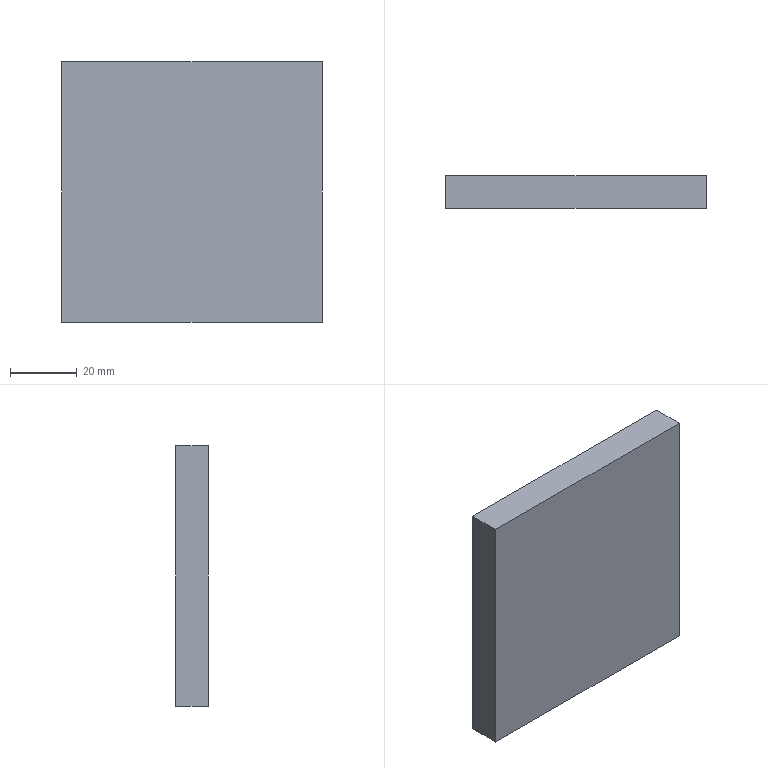Part | STEP file | 1 solid | 6 faces | box 77.948 x 9.733 x 78 mm | volume 59173 mm3 | plane 6
STEP:
#1=CARTESIAN_POINT('',(0.,0.,0.));
#2=DIRECTION('',(0.,0.,1.));
#3=DIRECTION('',(1.,0.,0.));
#4=AXIS2_PLACEMENT_3D('',#1,#2,#3);
#5=CARTESIAN_POINT('',(302.229,744.522,117.013));
#6=VERTEX_POINT('',#5);
#7=CARTESIAN_POINT('',(302.229,734.79,117.013));
#8=VERTEX_POINT('',#7);
#9=CARTESIAN_POINT('',(302.229,0.,117.013));
#10=DIRECTION('',(0.,-1.,0.));
#11=VECTOR('',#10,1.);
#12=LINE('',#9,#11);
#13=CARTESIAN_POINT('',(302.229,734.79,195.013));
#14=DIRECTION('',(1.,0.,0.));
#15=DIRECTION('',(0.,0.,-1.));
#16=AXIS2_PLACEMENT_3D('',#13,#14,#15);
#17=PLANE('',#16);
#18=CARTESIAN_POINT('',(78.,-734.79));
#19=DIRECTION('',(0.,-1.));
#20=VECTOR('',#19,1.);
#21=LINE('',#18,#20);
#22=(GEOMETRIC_REPRESENTATION_CONTEXT(2)PARAMETRIC_REPRESENTATION_CONTEXT()REPRESENTATION_CONTEXT('',''));
#23=DEFINITIONAL_REPRESENTATION('',(#21),#22);
#24=PCURVE('',#17,#23);
#25=CARTESIAN_POINT('',(0.,0.,117.013));
#26=DIRECTION('',(0.,0.,-1.));
#27=DIRECTION('',(-1.,0.,0.));
#28=AXIS2_PLACEMENT_3D('',#25,#26,#27);
#29=PLANE('',#28);
#30=CARTESIAN_POINT('',(-302.229,0.));
#31=DIRECTION('',(0.,-1.));
#32=VECTOR('',#31,1.);
#33=LINE('',#30,#32);
#34=(GEOMETRIC_REPRESENTATION_CONTEXT(2)PARAMETRIC_REPRESENTATION_CONTEXT()REPRESENTATION_CONTEXT('',''));
#35=DEFINITIONAL_REPRESENTATION('',(#33),#34);
#36=PCURVE('',#29,#35);
#37=SURFACE_CURVE('',#12,(#24,#36),.PCURVE_S1.);
#38=EDGE_CURVE('',#6,#8,#37,.T.);
#39=ORIENTED_EDGE('',*,*,#38,.T.);
#40=CARTESIAN_POINT('',(302.229,734.79,195.013));
#41=VERTEX_POINT('',#40);
#42=CARTESIAN_POINT('',(302.229,734.79,195.013));
#43=DIRECTION('',(0.,0.,-1.));
#44=VECTOR('',#43,1.);
#45=LINE('',#42,#44);
#46=CARTESIAN_POINT('',(0.,0.));
#47=DIRECTION('',(1.,0.));
#48=VECTOR('',#47,1.);
#49=LINE('',#46,#48);
#50=(GEOMETRIC_REPRESENTATION_CONTEXT(2)PARAMETRIC_REPRESENTATION_CONTEXT()REPRESENTATION_CONTEXT('',''));
#51=DEFINITIONAL_REPRESENTATION('',(#49),#50);
#52=PCURVE('',#17,#51);
#53=CARTESIAN_POINT('',(317.229,734.79,195.013));
#54=DIRECTION('',(0.,1.,0.));
#55=DIRECTION('',(0.,0.,1.));
#56=AXIS2_PLACEMENT_3D('',#53,#54,#55);
#57=PLANE('',#56);
#58=CARTESIAN_POINT('',(0.,-15.));
#59=DIRECTION('',(-1.,0.));
#60=VECTOR('',#59,1.);
#61=LINE('',#58,#60);
#62=(GEOMETRIC_REPRESENTATION_CONTEXT(2)PARAMETRIC_REPRESENTATION_CONTEXT()REPRESENTATION_CONTEXT('',''));
#63=DEFINITIONAL_REPRESENTATION('',(#61),#62);
#64=PCURVE('',#57,#63);
#65=SURFACE_CURVE('',#45,(#52,#64),.PCURVE_S1.);
#66=EDGE_CURVE('',#41,#8,#65,.T.);
#67=ORIENTED_EDGE('',*,*,#66,.F.);
#68=CARTESIAN_POINT('',(302.229,744.522,195.013));
#69=VERTEX_POINT('',#68);
#70=CARTESIAN_POINT('',(302.229,0.,195.013));
#71=DIRECTION('',(0.,-1.,0.));
#72=VECTOR('',#71,1.);
#73=LINE('',#70,#72);
#74=CARTESIAN_POINT('',(0.,-734.79));
#75=DIRECTION('',(0.,-1.));
#76=VECTOR('',#75,1.);
#77=LINE('',#74,#76);
#78=(GEOMETRIC_REPRESENTATION_CONTEXT(2)PARAMETRIC_REPRESENTATION_CONTEXT()REPRESENTATION_CONTEXT('',''));
#79=DEFINITIONAL_REPRESENTATION('',(#77),#78);
#80=PCURVE('',#17,#79);
#81=CARTESIAN_POINT('',(0.,0.,195.013));
#82=DIRECTION('',(0.,0.,-1.));
#83=DIRECTION('',(-1.,0.,0.));
#84=AXIS2_PLACEMENT_3D('',#81,#82,#83);
#85=PLANE('',#84);
#86=CARTESIAN_POINT('',(-302.229,0.));
#87=DIRECTION('',(0.,-1.));
#88=VECTOR('',#87,1.);
#89=LINE('',#86,#88);
#90=(GEOMETRIC_REPRESENTATION_CONTEXT(2)PARAMETRIC_REPRESENTATION_CONTEXT()REPRESENTATION_CONTEXT('',''));
#91=DEFINITIONAL_REPRESENTATION('',(#89),#90);
#92=PCURVE('',#85,#91);
#93=SURFACE_CURVE('',#73,(#80,#92),.PCURVE_S1.);
#94=EDGE_CURVE('',#69,#41,#93,.T.);
#95=ORIENTED_EDGE('',*,*,#94,.F.);
#96=CARTESIAN_POINT('',(302.229,744.522,195.013));
#97=DIRECTION('',(0.,0.,-1.));
#98=VECTOR('',#97,1.);
#99=LINE('',#96,#98);
#100=CARTESIAN_POINT('',(0.,9.733));
#101=DIRECTION('',(1.,0.));
#102=VECTOR('',#101,1.);
#103=LINE('',#100,#102);
#104=(GEOMETRIC_REPRESENTATION_CONTEXT(2)PARAMETRIC_REPRESENTATION_CONTEXT()REPRESENTATION_CONTEXT('',''));
#105=DEFINITIONAL_REPRESENTATION('',(#103),#104);
#106=PCURVE('',#17,#105);
#107=CARTESIAN_POINT('',(317.229,744.522,195.013));
#108=DIRECTION('',(0.,-1.,0.));
#109=DIRECTION('',(0.,0.,-1.));
#110=AXIS2_PLACEMENT_3D('',#107,#108,#109);
#111=PLANE('',#110);
#112=CARTESIAN_POINT('',(0.,-15.));
#113=DIRECTION('',(1.,0.));
#114=VECTOR('',#113,1.);
#115=LINE('',#112,#114);
#116=(GEOMETRIC_REPRESENTATION_CONTEXT(2)PARAMETRIC_REPRESENTATION_CONTEXT()REPRESENTATION_CONTEXT('',''));
#117=DEFINITIONAL_REPRESENTATION('',(#115),#116);
#118=PCURVE('',#111,#117);
#119=SURFACE_CURVE('',#99,(#106,#118),.PCURVE_S1.);
#120=EDGE_CURVE('',#69,#6,#119,.T.);
#121=ORIENTED_EDGE('',*,*,#120,.T.);
#122=EDGE_LOOP('',(#39,#67,#95,#121));
#123=FACE_BOUND('',#122,.T.);
#124=ADVANCED_FACE('',(#123),#17,.F.);
#125=CARTESIAN_POINT('',(380.177,734.79,117.013));
#126=VERTEX_POINT('',#125);
#127=CARTESIAN_POINT('',(0.,734.79,117.013));
#128=DIRECTION('',(1.,0.,0.));
#129=VECTOR('',#128,1.);
#130=LINE('',#127,#129);
#131=CARTESIAN_POINT('',(-78.,-317.229));
#132=DIRECTION('',(0.,1.));
#133=VECTOR('',#132,1.);
#134=LINE('',#131,#133);
#135=(GEOMETRIC_REPRESENTATION_CONTEXT(2)PARAMETRIC_REPRESENTATION_CONTEXT()REPRESENTATION_CONTEXT('',''));
#136=DEFINITIONAL_REPRESENTATION('',(#134),#135);
#137=PCURVE('',#57,#136);
#138=CARTESIAN_POINT('',(0.,734.79));
#139=DIRECTION('',(-1.,0.));
#140=VECTOR('',#139,1.);
#141=LINE('',#138,#140);
#142=(GEOMETRIC_REPRESENTATION_CONTEXT(2)PARAMETRIC_REPRESENTATION_CONTEXT()REPRESENTATION_CONTEXT('',''));
#143=DEFINITIONAL_REPRESENTATION('',(#141),#142);
#144=PCURVE('',#29,#143);
#145=SURFACE_CURVE('',#130,(#137,#144),.PCURVE_S1.);
#146=EDGE_CURVE('',#8,#126,#145,.T.);
#147=ORIENTED_EDGE('',*,*,#146,.T.);
#148=CARTESIAN_POINT('',(380.177,734.79,195.013));
#149=VERTEX_POINT('',#148);
#150=CARTESIAN_POINT('',(380.177,734.79,195.013));
#151=DIRECTION('',(0.,0.,-1.));
#152=VECTOR('',#151,1.);
#153=LINE('',#150,#152);
#154=CARTESIAN_POINT('',(0.,62.948));
#155=DIRECTION('',(-1.,0.));
#156=VECTOR('',#155,1.);
#157=LINE('',#154,#156);
#158=(GEOMETRIC_REPRESENTATION_CONTEXT(2)PARAMETRIC_REPRESENTATION_CONTEXT()REPRESENTATION_CONTEXT('',''));
#159=DEFINITIONAL_REPRESENTATION('',(#157),#158);
#160=PCURVE('',#57,#159);
#161=CARTESIAN_POINT('',(380.177,734.79,195.013));
#162=DIRECTION('',(-1.,0.,0.));
#163=DIRECTION('',(0.,0.,1.));
#164=AXIS2_PLACEMENT_3D('',#161,#162,#163);
#165=PLANE('',#164);
#166=CARTESIAN_POINT('',(0.,0.));
#167=DIRECTION('',(-1.,0.));
#168=VECTOR('',#167,1.);
#169=LINE('',#166,#168);
#170=(GEOMETRIC_REPRESENTATION_CONTEXT(2)PARAMETRIC_REPRESENTATION_CONTEXT()REPRESENTATION_CONTEXT('',''));
#171=DEFINITIONAL_REPRESENTATION('',(#169),#170);
#172=PCURVE('',#165,#171);
#173=SURFACE_CURVE('',#153,(#160,#172),.PCURVE_S1.);
#174=EDGE_CURVE('',#149,#126,#173,.T.);
#175=ORIENTED_EDGE('',*,*,#174,.F.);
#176=CARTESIAN_POINT('',(317.229,734.79,195.013));
#177=DIRECTION('',(1.,0.,0.));
#178=VECTOR('',#177,1.);
#179=LINE('',#176,#178);
#180=CARTESIAN_POINT('',(0.,0.));
#181=DIRECTION('',(0.,1.));
#182=VECTOR('',#181,1.);
#183=LINE('',#180,#182);
#184=(GEOMETRIC_REPRESENTATION_CONTEXT(2)PARAMETRIC_REPRESENTATION_CONTEXT()REPRESENTATION_CONTEXT('',''));
#185=DEFINITIONAL_REPRESENTATION('',(#183),#184);
#186=PCURVE('',#57,#185);
#187=CARTESIAN_POINT('',(-317.229,734.79));
#188=DIRECTION('',(-1.,0.));
#189=VECTOR('',#188,1.);
#190=LINE('',#187,#189);
#191=(GEOMETRIC_REPRESENTATION_CONTEXT(2)PARAMETRIC_REPRESENTATION_CONTEXT()REPRESENTATION_CONTEXT('',''));
#192=DEFINITIONAL_REPRESENTATION('',(#190),#191);
#193=PCURVE('',#85,#192);
#194=SURFACE_CURVE('',#179,(#186,#193),.PCURVE_S1.);
#195=EDGE_CURVE('',#41,#149,#194,.T.);
#196=ORIENTED_EDGE('',*,*,#195,.F.);
#197=ORIENTED_EDGE('',*,*,#66,.T.);
#198=EDGE_LOOP('',(#147,#175,#196,#197));
#199=FACE_BOUND('',#198,.T.);
#200=ADVANCED_FACE('',(#199),#57,.F.);
#201=CARTESIAN_POINT('',(380.177,744.522,117.013));
#202=VERTEX_POINT('',#201);
#203=CARTESIAN_POINT('',(380.177,0.,117.013));
#204=DIRECTION('',(0.,1.,0.));
#205=VECTOR('',#204,1.);
#206=LINE('',#203,#205);
#207=CARTESIAN_POINT('',(-78.,-734.79));
#208=DIRECTION('',(0.,1.));
#209=VECTOR('',#208,1.);
#210=LINE('',#207,#209);
#211=(GEOMETRIC_REPRESENTATION_CONTEXT(2)PARAMETRIC_REPRESENTATION_CONTEXT()REPRESENTATION_CONTEXT('',''));
#212=DEFINITIONAL_REPRESENTATION('',(#210),#211);
#213=PCURVE('',#165,#212);
#214=CARTESIAN_POINT('',(-380.177,0.));
#215=DIRECTION('',(0.,1.));
#216=VECTOR('',#215,1.);
#217=LINE('',#214,#216);
#218=(GEOMETRIC_REPRESENTATION_CONTEXT(2)PARAMETRIC_REPRESENTATION_CONTEXT()REPRESENTATION_CONTEXT('',''));
#219=DEFINITIONAL_REPRESENTATION('',(#217),#218);
#220=PCURVE('',#29,#219);
#221=SURFACE_CURVE('',#206,(#213,#220),.PCURVE_S1.);
#222=EDGE_CURVE('',#126,#202,#221,.T.);
#223=ORIENTED_EDGE('',*,*,#222,.T.);
#224=CARTESIAN_POINT('',(380.177,744.522,195.013));
#225=VERTEX_POINT('',#224);
#226=CARTESIAN_POINT('',(380.177,744.522,195.013));
#227=DIRECTION('',(0.,0.,-1.));
#228=VECTOR('',#227,1.);
#229=LINE('',#226,#228);
#230=CARTESIAN_POINT('',(0.,9.733));
#231=DIRECTION('',(-1.,0.));
#232=VECTOR('',#231,1.);
#233=LINE('',#230,#232);
#234=(GEOMETRIC_REPRESENTATION_CONTEXT(2)PARAMETRIC_REPRESENTATION_CONTEXT()REPRESENTATION_CONTEXT('',''));
#235=DEFINITIONAL_REPRESENTATION('',(#233),#234);
#236=PCURVE('',#165,#235);
#237=CARTESIAN_POINT('',(0.,62.948));
#238=DIRECTION('',(1.,0.));
#239=VECTOR('',#238,1.);
#240=LINE('',#237,#239);
#241=(GEOMETRIC_REPRESENTATION_CONTEXT(2)PARAMETRIC_REPRESENTATION_CONTEXT()REPRESENTATION_CONTEXT('',''));
#242=DEFINITIONAL_REPRESENTATION('',(#240),#241);
#243=PCURVE('',#111,#242);
#244=SURFACE_CURVE('',#229,(#236,#243),.PCURVE_S1.);
#245=EDGE_CURVE('',#225,#202,#244,.T.);
#246=ORIENTED_EDGE('',*,*,#245,.F.);
#247=CARTESIAN_POINT('',(380.177,0.,195.013));
#248=DIRECTION('',(0.,1.,0.));
#249=VECTOR('',#248,1.);
#250=LINE('',#247,#249);
#251=CARTESIAN_POINT('',(0.,-734.79));
#252=DIRECTION('',(0.,1.));
#253=VECTOR('',#252,1.);
#254=LINE('',#251,#253);
#255=(GEOMETRIC_REPRESENTATION_CONTEXT(2)PARAMETRIC_REPRESENTATION_CONTEXT()REPRESENTATION_CONTEXT('',''));
#256=DEFINITIONAL_REPRESENTATION('',(#254),#255);
#257=PCURVE('',#165,#256);
#258=CARTESIAN_POINT('',(-380.177,0.));
#259=DIRECTION('',(0.,1.));
#260=VECTOR('',#259,1.);
#261=LINE('',#258,#260);
#262=(GEOMETRIC_REPRESENTATION_CONTEXT(2)PARAMETRIC_REPRESENTATION_CONTEXT()REPRESENTATION_CONTEXT('',''));
#263=DEFINITIONAL_REPRESENTATION('',(#261),#262);
#264=PCURVE('',#85,#263);
#265=SURFACE_CURVE('',#250,(#257,#264),.PCURVE_S1.);
#266=EDGE_CURVE('',#149,#225,#265,.T.);
#267=ORIENTED_EDGE('',*,*,#266,.F.);
#268=ORIENTED_EDGE('',*,*,#174,.T.);
#269=EDGE_LOOP('',(#223,#246,#267,#268));
#270=FACE_BOUND('',#269,.T.);
#271=ADVANCED_FACE('',(#270),#165,.F.);
#272=CARTESIAN_POINT('',(0.,744.522,117.013));
#273=DIRECTION('',(-1.,0.,0.));
#274=VECTOR('',#273,1.);
#275=LINE('',#272,#274);
#276=CARTESIAN_POINT('',(78.,-317.229));
#277=DIRECTION('',(0.,-1.));
#278=VECTOR('',#277,1.);
#279=LINE('',#276,#278);
#280=(GEOMETRIC_REPRESENTATION_CONTEXT(2)PARAMETRIC_REPRESENTATION_CONTEXT()REPRESENTATION_CONTEXT('',''));
#281=DEFINITIONAL_REPRESENTATION('',(#279),#280);
#282=PCURVE('',#111,#281);
#283=CARTESIAN_POINT('',(0.,744.522));
#284=DIRECTION('',(1.,0.));
#285=VECTOR('',#284,1.);
#286=LINE('',#283,#285);
#287=(GEOMETRIC_REPRESENTATION_CONTEXT(2)PARAMETRIC_REPRESENTATION_CONTEXT()REPRESENTATION_CONTEXT('',''));
#288=DEFINITIONAL_REPRESENTATION('',(#286),#287);
#289=PCURVE('',#29,#288);
#290=SURFACE_CURVE('',#275,(#282,#289),.PCURVE_S1.);
#291=EDGE_CURVE('',#202,#6,#290,.T.);
#292=ORIENTED_EDGE('',*,*,#291,.T.);
#293=ORIENTED_EDGE('',*,*,#120,.F.);
#294=CARTESIAN_POINT('',(0.,744.522,195.013));
#295=DIRECTION('',(-1.,0.,0.));
#296=VECTOR('',#295,1.);
#297=LINE('',#294,#296);
#298=CARTESIAN_POINT('',(0.,-317.229));
#299=DIRECTION('',(0.,-1.));
#300=VECTOR('',#299,1.);
#301=LINE('',#298,#300);
#302=(GEOMETRIC_REPRESENTATION_CONTEXT(2)PARAMETRIC_REPRESENTATION_CONTEXT()REPRESENTATION_CONTEXT('',''));
#303=DEFINITIONAL_REPRESENTATION('',(#301),#302);
#304=PCURVE('',#111,#303);
#305=CARTESIAN_POINT('',(0.,744.522));
#306=DIRECTION('',(1.,0.));
#307=VECTOR('',#306,1.);
#308=LINE('',#305,#307);
#309=(GEOMETRIC_REPRESENTATION_CONTEXT(2)PARAMETRIC_REPRESENTATION_CONTEXT()REPRESENTATION_CONTEXT('',''));
#310=DEFINITIONAL_REPRESENTATION('',(#308),#309);
#311=PCURVE('',#85,#310);
#312=SURFACE_CURVE('',#297,(#304,#311),.PCURVE_S1.);
#313=EDGE_CURVE('',#225,#69,#312,.T.);
#314=ORIENTED_EDGE('',*,*,#313,.F.);
#315=ORIENTED_EDGE('',*,*,#245,.T.);
#316=EDGE_LOOP('',(#292,#293,#314,#315));
#317=FACE_BOUND('',#316,.T.);
#318=ADVANCED_FACE('',(#317),#111,.F.);
#319=ORIENTED_EDGE('',*,*,#94,.T.);
#320=ORIENTED_EDGE('',*,*,#195,.T.);
#321=ORIENTED_EDGE('',*,*,#266,.T.);
#322=ORIENTED_EDGE('',*,*,#313,.T.);
#323=EDGE_LOOP('',(#319,#320,#321,#322));
#324=FACE_BOUND('',#323,.T.);
#325=ADVANCED_FACE('',(#324),#85,.F.);
#326=ORIENTED_EDGE('',*,*,#38,.F.);
#327=ORIENTED_EDGE('',*,*,#291,.F.);
#328=ORIENTED_EDGE('',*,*,#222,.F.);
#329=ORIENTED_EDGE('',*,*,#146,.F.);
#330=EDGE_LOOP('',(#326,#327,#328,#329));
#331=FACE_BOUND('',#330,.T.);
#332=ADVANCED_FACE('',(#331),#29,.T.);
#333=CLOSED_SHELL('',(#124,#200,#271,#318,#325,#332));
#334=MANIFOLD_SOLID_BREP('',#333);
#335=(LENGTH_UNIT()NAMED_UNIT(*)SI_UNIT(.MILLI.,.METRE.));
#336=UNCERTAINTY_MEASURE_WITH_UNIT(LENGTH_MEASURE(0.0000001),#335,'','');
#337=(NAMED_UNIT(*)PLANE_ANGLE_UNIT()SI_UNIT($,.RADIAN.));
#338=(NAMED_UNIT(*)SI_UNIT($,.STERADIAN.)SOLID_ANGLE_UNIT());
#339=(GEOMETRIC_REPRESENTATION_CONTEXT(3)GLOBAL_UNCERTAINTY_ASSIGNED_CONTEXT((#336))GLOBAL_UNIT_ASSIGNED_CONTEXT((#335,#337,#338))REPRESENTATION_CONTEXT('',''));
#340=ADVANCED_BREP_SHAPE_REPRESENTATION('',(#4,#334),#339);